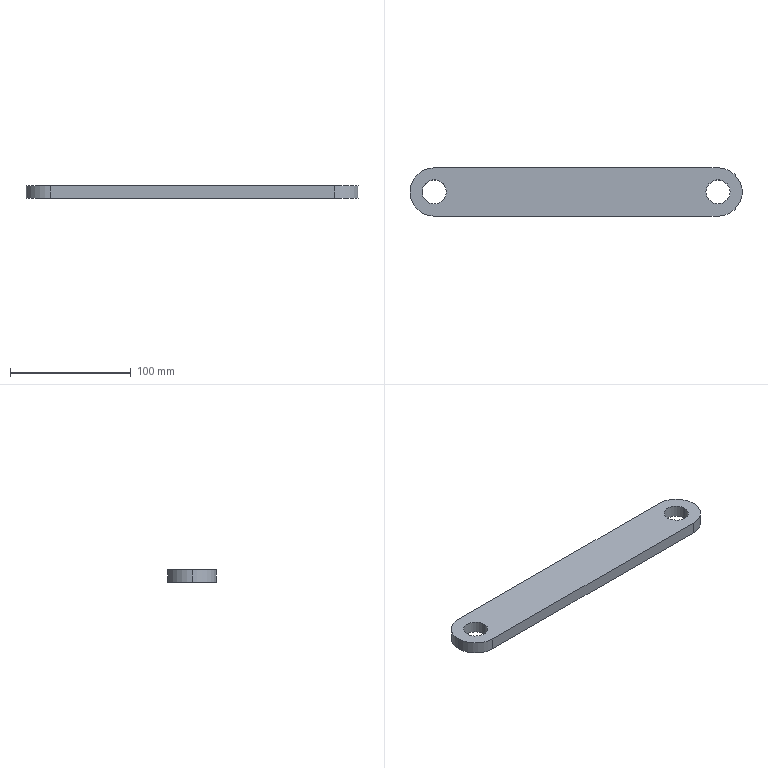Part | SolidWorks | features Extrusion 1, ICE 1 | 1 solid | 11 faces | box 275 x 40 x 10 mm | volume 100283 mm3 | cylinder 7 | plane 4 | commonest cylinder face diameters 20 x4 40 x3
STEP:
#1=CARTESIAN_POINT('',(-127.5,0.,0.));
#2=VERTEX_POINT('',#1);
#3=CARTESIAN_POINT('',(-107.5,0.,0.));
#4=VERTEX_POINT('',#3);
#5=CARTESIAN_POINT('',(-117.5,0.,0.));
#6=DIRECTION('',(0.,0.,1.));
#7=DIRECTION('',(1.,0.,0.));
#8=AXIS2_PLACEMENT_3D('',#5,#6,#7);
#9=CIRCLE('',#8,10.);
#10=EDGE_CURVE('',#2,#4,#9,.T.);
#11=ORIENTED_EDGE('',*,*,#10,.F.);
#12=CARTESIAN_POINT('',(-127.5,0.,10.));
#13=VERTEX_POINT('',#12);
#14=CARTESIAN_POINT('',(-127.5,0.,0.));
#15=DIRECTION('',(0.,0.,1.));
#16=VECTOR('',#15,1000.);
#17=LINE('',#14,#16);
#18=EDGE_CURVE('',#2,#13,#17,.T.);
#19=ORIENTED_EDGE('',*,*,#18,.T.);
#20=CARTESIAN_POINT('',(-107.5,0.,10.));
#21=VERTEX_POINT('',#20);
#22=CARTESIAN_POINT('',(-117.5,0.,10.));
#23=DIRECTION('',(0.,0.,1.));
#24=DIRECTION('',(1.,0.,0.));
#25=AXIS2_PLACEMENT_3D('',#22,#23,#24);
#26=CIRCLE('',#25,10.);
#27=EDGE_CURVE('',#13,#21,#26,.T.);
#28=ORIENTED_EDGE('',*,*,#27,.T.);
#29=CARTESIAN_POINT('',(-107.5,0.,0.));
#30=DIRECTION('',(0.,0.,1.));
#31=VECTOR('',#30,1000.);
#32=LINE('',#29,#31);
#33=EDGE_CURVE('',#4,#21,#32,.T.);
#34=ORIENTED_EDGE('',*,*,#33,.F.);
#35=EDGE_LOOP('',(#11,#19,#28,#34));
#36=FACE_OUTER_BOUND('',#35,.T.);
#37=CARTESIAN_POINT('',(-117.5,0.,0.));
#38=DIRECTION('',(0.,0.,1.));
#39=DIRECTION('',(1.,0.,0.));
#40=AXIS2_PLACEMENT_3D('',#37,#38,#39);
#41=CYLINDRICAL_SURFACE('',#40,10.);
#42=ADVANCED_FACE('',(#36),#41,.F.);
#43=CARTESIAN_POINT('',(107.5,0.,0.));
#44=VERTEX_POINT('',#43);
#45=CARTESIAN_POINT('',(127.5,0.,0.));
#46=VERTEX_POINT('',#45);
#47=CARTESIAN_POINT('',(117.5,0.,0.));
#48=DIRECTION('',(0.,0.,1.));
#49=DIRECTION('',(1.,0.,0.));
#50=AXIS2_PLACEMENT_3D('',#47,#48,#49);
#51=CIRCLE('',#50,10.);
#52=EDGE_CURVE('',#44,#46,#51,.T.);
#53=ORIENTED_EDGE('',*,*,#52,.F.);
#54=CARTESIAN_POINT('',(107.5,0.,10.));
#55=VERTEX_POINT('',#54);
#56=CARTESIAN_POINT('',(107.5,0.,0.));
#57=DIRECTION('',(0.,0.,1.));
#58=VECTOR('',#57,1000.);
#59=LINE('',#56,#58);
#60=EDGE_CURVE('',#44,#55,#59,.T.);
#61=ORIENTED_EDGE('',*,*,#60,.T.);
#62=CARTESIAN_POINT('',(127.5,0.,10.));
#63=VERTEX_POINT('',#62);
#64=CARTESIAN_POINT('',(117.5,0.,10.));
#65=DIRECTION('',(0.,0.,1.));
#66=DIRECTION('',(1.,0.,0.));
#67=AXIS2_PLACEMENT_3D('',#64,#65,#66);
#68=CIRCLE('',#67,10.);
#69=EDGE_CURVE('',#55,#63,#68,.T.);
#70=ORIENTED_EDGE('',*,*,#69,.T.);
#71=CARTESIAN_POINT('',(127.5,0.,0.));
#72=DIRECTION('',(0.,0.,1.));
#73=VECTOR('',#72,1000.);
#74=LINE('',#71,#73);
#75=EDGE_CURVE('',#46,#63,#74,.T.);
#76=ORIENTED_EDGE('',*,*,#75,.F.);
#77=EDGE_LOOP('',(#53,#61,#70,#76));
#78=FACE_OUTER_BOUND('',#77,.T.);
#79=CARTESIAN_POINT('',(117.5,0.,0.));
#80=DIRECTION('',(0.,0.,1.));
#81=DIRECTION('',(1.,0.,0.));
#82=AXIS2_PLACEMENT_3D('',#79,#80,#81);
#83=CYLINDRICAL_SURFACE('',#82,10.);
#84=ADVANCED_FACE('',(#78),#83,.F.);
#85=CARTESIAN_POINT('',(-137.5,0.,10.));
#86=VERTEX_POINT('',#85);
#87=CARTESIAN_POINT('',(-117.5,-20.,10.));
#88=VERTEX_POINT('',#87);
#89=CARTESIAN_POINT('',(-117.5,0.,10.));
#90=DIRECTION('',(0.,0.,1.));
#91=DIRECTION('',(1.,0.,0.));
#92=AXIS2_PLACEMENT_3D('',#89,#90,#91);
#93=CIRCLE('',#92,20.);
#94=EDGE_CURVE('',#86,#88,#93,.T.);
#95=ORIENTED_EDGE('',*,*,#94,.F.);
#96=CARTESIAN_POINT('',(-137.5,0.,0.));
#97=VERTEX_POINT('',#96);
#98=CARTESIAN_POINT('',(-137.5,0.,10.));
#99=DIRECTION('',(0.,0.,-1.));
#100=VECTOR('',#99,1000.);
#101=LINE('',#98,#100);
#102=EDGE_CURVE('',#86,#97,#101,.T.);
#103=ORIENTED_EDGE('',*,*,#102,.T.);
#104=CARTESIAN_POINT('',(-117.5,-20.,0.));
#105=VERTEX_POINT('',#104);
#106=CARTESIAN_POINT('',(-117.5,0.,0.));
#107=DIRECTION('',(0.,0.,1.));
#108=DIRECTION('',(1.,0.,0.));
#109=AXIS2_PLACEMENT_3D('',#106,#107,#108);
#110=CIRCLE('',#109,20.);
#111=EDGE_CURVE('',#97,#105,#110,.T.);
#112=ORIENTED_EDGE('',*,*,#111,.T.);
#113=CARTESIAN_POINT('',(-117.5,-20.,10.));
#114=DIRECTION('',(0.,0.,-1.));
#115=VECTOR('',#114,1000.);
#116=LINE('',#113,#115);
#117=EDGE_CURVE('',#88,#105,#116,.T.);
#118=ORIENTED_EDGE('',*,*,#117,.F.);
#119=EDGE_LOOP('',(#95,#103,#112,#118));
#120=FACE_OUTER_BOUND('',#119,.T.);
#121=CARTESIAN_POINT('',(-117.5,0.,10.));
#122=DIRECTION('',(0.,0.,-1.));
#123=DIRECTION('',(-1.,0.,0.));
#124=AXIS2_PLACEMENT_3D('',#121,#122,#123);
#125=CYLINDRICAL_SURFACE('',#124,20.);
#126=ADVANCED_FACE('',(#120),#125,.T.);
#127=ORIENTED_EDGE('',*,*,#102,.F.);
#128=CARTESIAN_POINT('',(-117.5,20.,10.));
#129=VERTEX_POINT('',#128);
#130=CARTESIAN_POINT('',(-117.5,0.,10.));
#131=DIRECTION('',(0.,0.,1.));
#132=DIRECTION('',(1.,0.,0.));
#133=AXIS2_PLACEMENT_3D('',#130,#131,#132);
#134=CIRCLE('',#133,20.);
#135=EDGE_CURVE('',#129,#86,#134,.T.);
#136=ORIENTED_EDGE('',*,*,#135,.F.);
#137=CARTESIAN_POINT('',(-117.5,20.,0.));
#138=VERTEX_POINT('',#137);
#139=CARTESIAN_POINT('',(-117.5,20.,10.));
#140=DIRECTION('',(0.,0.,-1.));
#141=VECTOR('',#140,1000.);
#142=LINE('',#139,#141);
#143=EDGE_CURVE('',#129,#138,#142,.T.);
#144=ORIENTED_EDGE('',*,*,#143,.T.);
#145=CARTESIAN_POINT('',(-117.5,0.,0.));
#146=DIRECTION('',(0.,0.,1.));
#147=DIRECTION('',(1.,0.,0.));
#148=AXIS2_PLACEMENT_3D('',#145,#146,#147);
#149=CIRCLE('',#148,20.);
#150=EDGE_CURVE('',#138,#97,#149,.T.);
#151=ORIENTED_EDGE('',*,*,#150,.T.);
#152=EDGE_LOOP('',(#127,#136,#144,#151));
#153=FACE_OUTER_BOUND('',#152,.T.);
#154=CARTESIAN_POINT('',(-117.5,0.,10.));
#155=DIRECTION('',(0.,0.,-1.));
#156=DIRECTION('',(-1.,0.,0.));
#157=AXIS2_PLACEMENT_3D('',#154,#155,#156);
#158=CYLINDRICAL_SURFACE('',#157,20.);
#159=ADVANCED_FACE('',(#153),#158,.T.);
#160=CARTESIAN_POINT('',(117.5,-20.,0.));
#161=VERTEX_POINT('',#160);
#162=CARTESIAN_POINT('',(-117.5,-20.,0.));
#163=DIRECTION('',(1.,0.,0.));
#164=VECTOR('',#163,1000.);
#165=LINE('',#162,#164);
#166=EDGE_CURVE('',#105,#161,#165,.T.);
#167=ORIENTED_EDGE('',*,*,#166,.T.);
#168=CARTESIAN_POINT('',(117.5,-20.,10.));
#169=VERTEX_POINT('',#168);
#170=CARTESIAN_POINT('',(117.5,-20.,10.));
#171=DIRECTION('',(0.,0.,-1.));
#172=VECTOR('',#171,1000.);
#173=LINE('',#170,#172);
#174=EDGE_CURVE('',#169,#161,#173,.T.);
#175=ORIENTED_EDGE('',*,*,#174,.F.);
#176=CARTESIAN_POINT('',(-117.5,-20.,10.));
#177=DIRECTION('',(1.,0.,0.));
#178=VECTOR('',#177,1000.);
#179=LINE('',#176,#178);
#180=EDGE_CURVE('',#88,#169,#179,.T.);
#181=ORIENTED_EDGE('',*,*,#180,.F.);
#182=ORIENTED_EDGE('',*,*,#117,.T.);
#183=EDGE_LOOP('',(#167,#175,#181,#182));
#184=FACE_OUTER_BOUND('',#183,.T.);
#185=CARTESIAN_POINT('',(-117.5,-20.,10.));
#186=DIRECTION('',(0.,1.,0.));
#187=DIRECTION('',(0.,0.,1.));
#188=AXIS2_PLACEMENT_3D('',#185,#186,#187);
#189=PLANE('',#188);
#190=ADVANCED_FACE('',(#184),#189,.F.);
#191=CARTESIAN_POINT('',(117.5,20.,0.));
#192=VERTEX_POINT('',#191);
#193=CARTESIAN_POINT('',(117.5,0.,0.));
#194=DIRECTION('',(0.,0.,1.));
#195=DIRECTION('',(1.,0.,0.));
#196=AXIS2_PLACEMENT_3D('',#193,#194,#195);
#197=CIRCLE('',#196,20.);
#198=EDGE_CURVE('',#161,#192,#197,.T.);
#199=ORIENTED_EDGE('',*,*,#198,.T.);
#200=CARTESIAN_POINT('',(117.5,20.,10.));
#201=VERTEX_POINT('',#200);
#202=CARTESIAN_POINT('',(117.5,20.,10.));
#203=DIRECTION('',(0.,0.,-1.));
#204=VECTOR('',#203,1000.);
#205=LINE('',#202,#204);
#206=EDGE_CURVE('',#201,#192,#205,.T.);
#207=ORIENTED_EDGE('',*,*,#206,.F.);
#208=CARTESIAN_POINT('',(117.5,0.,10.));
#209=DIRECTION('',(0.,0.,1.));
#210=DIRECTION('',(1.,0.,0.));
#211=AXIS2_PLACEMENT_3D('',#208,#209,#210);
#212=CIRCLE('',#211,20.);
#213=EDGE_CURVE('',#169,#201,#212,.T.);
#214=ORIENTED_EDGE('',*,*,#213,.F.);
#215=ORIENTED_EDGE('',*,*,#174,.T.);
#216=EDGE_LOOP('',(#199,#207,#214,#215));
#217=FACE_OUTER_BOUND('',#216,.T.);
#218=CARTESIAN_POINT('',(117.5,0.,10.));
#219=DIRECTION('',(0.,0.,-1.));
#220=DIRECTION('',(-1.,0.,0.));
#221=AXIS2_PLACEMENT_3D('',#218,#219,#220);
#222=CYLINDRICAL_SURFACE('',#221,20.);
#223=ADVANCED_FACE('',(#217),#222,.T.);
#224=CARTESIAN_POINT('',(-117.5,20.,0.));
#225=DIRECTION('',(-1.,0.,0.));
#226=VECTOR('',#225,1000.);
#227=LINE('',#224,#226);
#228=EDGE_CURVE('',#192,#138,#227,.T.);
#229=ORIENTED_EDGE('',*,*,#228,.T.);
#230=ORIENTED_EDGE('',*,*,#143,.F.);
#231=CARTESIAN_POINT('',(-117.5,20.,10.));
#232=DIRECTION('',(-1.,0.,0.));
#233=VECTOR('',#232,1000.);
#234=LINE('',#231,#233);
#235=EDGE_CURVE('',#201,#129,#234,.T.);
#236=ORIENTED_EDGE('',*,*,#235,.F.);
#237=ORIENTED_EDGE('',*,*,#206,.T.);
#238=EDGE_LOOP('',(#229,#230,#236,#237));
#239=FACE_OUTER_BOUND('',#238,.T.);
#240=CARTESIAN_POINT('',(-117.5,20.,10.));
#241=DIRECTION('',(0.,-1.,0.));
#242=DIRECTION('',(1.,0.,0.));
#243=AXIS2_PLACEMENT_3D('',#240,#241,#242);
#244=PLANE('',#243);
#245=ADVANCED_FACE('',(#239),#244,.F.);
#246=CARTESIAN_POINT('',(-117.5,0.,10.));
#247=DIRECTION('',(0.,0.,1.));
#248=DIRECTION('',(1.,0.,0.));
#249=AXIS2_PLACEMENT_3D('',#246,#247,#248);
#250=CIRCLE('',#249,10.);
#251=EDGE_CURVE('',#21,#13,#250,.T.);
#252=ORIENTED_EDGE('',*,*,#251,.F.);
#253=ORIENTED_EDGE('',*,*,#27,.F.);
#254=EDGE_LOOP('',(#252,#253));
#255=FACE_BOUND('',#254,.T.);
#256=CARTESIAN_POINT('',(117.5,0.,10.));
#257=DIRECTION('',(0.,0.,1.));
#258=DIRECTION('',(1.,0.,0.));
#259=AXIS2_PLACEMENT_3D('',#256,#257,#258);
#260=CIRCLE('',#259,10.);
#261=EDGE_CURVE('',#63,#55,#260,.T.);
#262=ORIENTED_EDGE('',*,*,#261,.F.);
#263=ORIENTED_EDGE('',*,*,#69,.F.);
#264=EDGE_LOOP('',(#262,#263));
#265=FACE_BOUND('',#264,.T.);
#266=ORIENTED_EDGE('',*,*,#135,.T.);
#267=ORIENTED_EDGE('',*,*,#94,.T.);
#268=ORIENTED_EDGE('',*,*,#180,.T.);
#269=ORIENTED_EDGE('',*,*,#213,.T.);
#270=ORIENTED_EDGE('',*,*,#235,.T.);
#271=EDGE_LOOP('',(#266,#267,#268,#269,#270));
#272=FACE_OUTER_BOUND('',#271,.T.);
#273=CARTESIAN_POINT('',(-117.5,0.,10.));
#274=DIRECTION('',(0.,0.,1.));
#275=DIRECTION('',(1.,0.,0.));
#276=AXIS2_PLACEMENT_3D('',#273,#274,#275);
#277=PLANE('',#276);
#278=ADVANCED_FACE('',(#255,#265,#272),#277,.T.);
#279=CARTESIAN_POINT('',(-117.5,0.,0.));
#280=DIRECTION('',(0.,0.,1.));
#281=DIRECTION('',(1.,0.,0.));
#282=AXIS2_PLACEMENT_3D('',#279,#280,#281);
#283=CIRCLE('',#282,10.);
#284=EDGE_CURVE('',#4,#2,#283,.T.);
#285=ORIENTED_EDGE('',*,*,#284,.T.);
#286=ORIENTED_EDGE('',*,*,#10,.T.);
#287=EDGE_LOOP('',(#285,#286));
#288=FACE_BOUND('',#287,.T.);
#289=CARTESIAN_POINT('',(117.5,0.,0.));
#290=DIRECTION('',(0.,0.,1.));
#291=DIRECTION('',(1.,0.,0.));
#292=AXIS2_PLACEMENT_3D('',#289,#290,#291);
#293=CIRCLE('',#292,10.);
#294=EDGE_CURVE('',#46,#44,#293,.T.);
#295=ORIENTED_EDGE('',*,*,#294,.T.);
#296=ORIENTED_EDGE('',*,*,#52,.T.);
#297=EDGE_LOOP('',(#295,#296));
#298=FACE_BOUND('',#297,.T.);
#299=ORIENTED_EDGE('',*,*,#150,.F.);
#300=ORIENTED_EDGE('',*,*,#228,.F.);
#301=ORIENTED_EDGE('',*,*,#198,.F.);
#302=ORIENTED_EDGE('',*,*,#166,.F.);
#303=ORIENTED_EDGE('',*,*,#111,.F.);
#304=EDGE_LOOP('',(#299,#300,#301,#302,#303));
#305=FACE_OUTER_BOUND('',#304,.T.);
#306=CARTESIAN_POINT('',(-117.5,0.,0.));
#307=DIRECTION('',(0.,0.,1.));
#308=DIRECTION('',(1.,0.,0.));
#309=AXIS2_PLACEMENT_3D('',#306,#307,#308);
#310=PLANE('',#309);
#311=ADVANCED_FACE('',(#288,#298,#305),#310,.F.);
#312=ORIENTED_EDGE('',*,*,#60,.F.);
#313=ORIENTED_EDGE('',*,*,#294,.F.);
#314=ORIENTED_EDGE('',*,*,#75,.T.);
#315=ORIENTED_EDGE('',*,*,#261,.T.);
#316=EDGE_LOOP('',(#312,#313,#314,#315));
#317=FACE_OUTER_BOUND('',#316,.T.);
#318=CARTESIAN_POINT('',(117.5,0.,0.));
#319=DIRECTION('',(0.,0.,1.));
#320=DIRECTION('',(1.,0.,0.));
#321=AXIS2_PLACEMENT_3D('',#318,#319,#320);
#322=CYLINDRICAL_SURFACE('',#321,10.);
#323=ADVANCED_FACE('',(#317),#322,.F.);
#324=ORIENTED_EDGE('',*,*,#18,.F.);
#325=ORIENTED_EDGE('',*,*,#284,.F.);
#326=ORIENTED_EDGE('',*,*,#33,.T.);
#327=ORIENTED_EDGE('',*,*,#251,.T.);
#328=EDGE_LOOP('',(#324,#325,#326,#327));
#329=FACE_OUTER_BOUND('',#328,.T.);
#330=CARTESIAN_POINT('',(-117.5,0.,0.));
#331=DIRECTION('',(0.,0.,1.));
#332=DIRECTION('',(1.,0.,0.));
#333=AXIS2_PLACEMENT_3D('',#330,#331,#332);
#334=CYLINDRICAL_SURFACE('',#333,10.);
#335=ADVANCED_FACE('',(#329),#334,.F.);
#336=CLOSED_SHELL('',(#42,#84,#126,#159,#190,#223,#245,#278,#311,#323,#335));
#337=MANIFOLD_SOLID_BREP('',#336);
#338=CARTESIAN_POINT('',(0.,0.,0.));
#339=DIRECTION('',(0.,0.,1.));
#340=DIRECTION('',(1.,0.,0.));
#341=AXIS2_PLACEMENT_3D('',#338,#339,#340);
#342=(LENGTH_UNIT()NAMED_UNIT(*)SI_UNIT(.MILLI.,.METRE.));
#343=UNCERTAINTY_MEASURE_WITH_UNIT(LENGTH_MEASURE(0.00001),#342,'','');
#344=(NAMED_UNIT(*)PLANE_ANGLE_UNIT()SI_UNIT($,.RADIAN.));
#345=(NAMED_UNIT(*)SI_UNIT($,.STERADIAN.)SOLID_ANGLE_UNIT());
#346=(GEOMETRIC_REPRESENTATION_CONTEXT(3)GLOBAL_UNCERTAINTY_ASSIGNED_CONTEXT((#343))GLOBAL_UNIT_ASSIGNED_CONTEXT((#342,#344,#345))REPRESENTATION_CONTEXT('',''));
#347=ADVANCED_BREP_SHAPE_REPRESENTATION('',(#337,#341),#346);